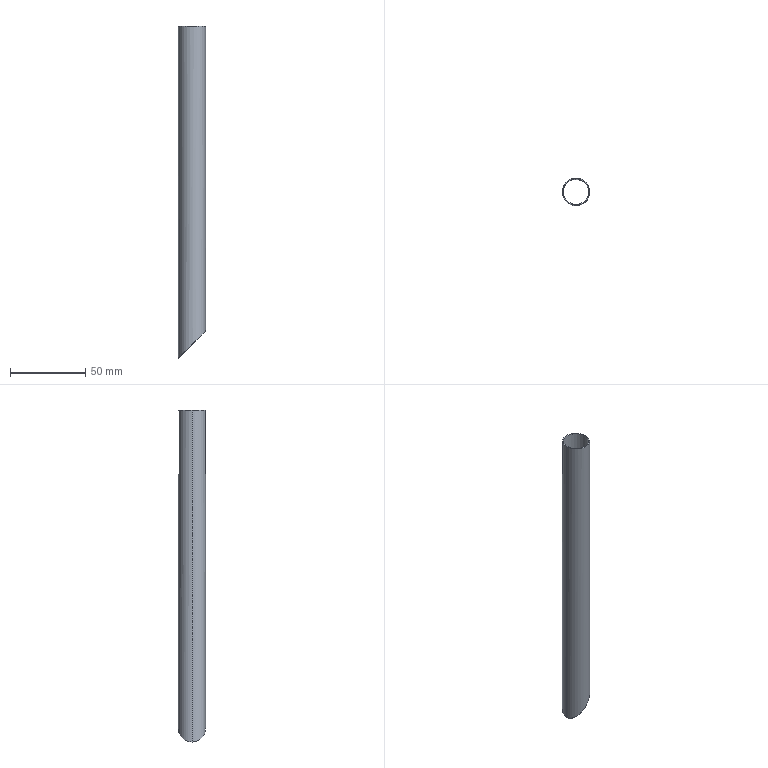Part | SolidWorks | features Extrusion 1, ICE 1 | 1 solid | 6 faces | box 18 x 18 x 220 mm | volume 5800 mm3 | cylinder 4 | plane 2 | commonest cylinder face diameters 17 x2 18 x2
STEP:
#1=CARTESIAN_POINT('',(-8.5,0.,220.));
#2=VERTEX_POINT('',#1);
#3=CARTESIAN_POINT('',(8.5,0.,220.));
#4=VERTEX_POINT('',#3);
#5=CARTESIAN_POINT('',(0.,0.,220.));
#6=DIRECTION('',(0.,0.,1.));
#7=DIRECTION('',(1.,0.,0.));
#8=AXIS2_PLACEMENT_3D('',#5,#6,#7);
#9=CIRCLE('',#8,8.5);
#10=EDGE_CURVE('',#2,#4,#9,.T.);
#11=ORIENTED_EDGE('',*,*,#10,.T.);
#12=CARTESIAN_POINT('',(8.5,0.,17.5));
#13=VERTEX_POINT('',#12);
#14=CARTESIAN_POINT('',(8.5,0.,220.));
#15=DIRECTION('',(0.,0.,-1.));
#16=VECTOR('',#15,1000.);
#17=LINE('',#14,#16);
#18=EDGE_CURVE('',#4,#13,#17,.T.);
#19=ORIENTED_EDGE('',*,*,#18,.T.);
#20=CARTESIAN_POINT('',(-8.5,0.,0.5));
#21=VERTEX_POINT('',#20);
#22=CARTESIAN_POINT('',(-8.5,0.,0.5));
#23=CARTESIAN_POINT('',(-8.5,-17.,0.5));
#24=CARTESIAN_POINT('',(8.5,-17.,17.5));
#25=CARTESIAN_POINT('',(8.5,0.,17.5));
#26=(BOUNDED_CURVE()B_SPLINE_CURVE(3,(#22,#23,#24,#25),.UNSPECIFIED.,.F.,.F.)B_SPLINE_CURVE_WITH_KNOTS((4,4),(0.,3.142),.UNSPECIFIED.)CURVE()GEOMETRIC_REPRESENTATION_ITEM()RATIONAL_B_SPLINE_CURVE((1.,0.3333,0.3333,1.))REPRESENTATION_ITEM(''));
#27=EDGE_CURVE('',#21,#13,#26,.T.);
#28=ORIENTED_EDGE('',*,*,#27,.F.);
#29=CARTESIAN_POINT('',(-8.5,0.,220.));
#30=DIRECTION('',(0.,0.,-1.));
#31=VECTOR('',#30,1000.);
#32=LINE('',#29,#31);
#33=EDGE_CURVE('',#2,#21,#32,.T.);
#34=ORIENTED_EDGE('',*,*,#33,.F.);
#35=EDGE_LOOP('',(#11,#19,#28,#34));
#36=FACE_OUTER_BOUND('',#35,.T.);
#37=CARTESIAN_POINT('',(0.,0.,220.));
#38=DIRECTION('',(0.,0.,-1.));
#39=DIRECTION('',(-1.,0.,0.));
#40=AXIS2_PLACEMENT_3D('',#37,#38,#39);
#41=CYLINDRICAL_SURFACE('',#40,8.5);
#42=ADVANCED_FACE('',(#36),#41,.F.);
#43=CARTESIAN_POINT('',(9.,0.,220.));
#44=VERTEX_POINT('',#43);
#45=CARTESIAN_POINT('',(-9.,0.,220.));
#46=VERTEX_POINT('',#45);
#47=CARTESIAN_POINT('',(0.,0.,220.));
#48=DIRECTION('',(0.,0.,1.));
#49=DIRECTION('',(1.,0.,0.));
#50=AXIS2_PLACEMENT_3D('',#47,#48,#49);
#51=CIRCLE('',#50,9.);
#52=EDGE_CURVE('',#44,#46,#51,.T.);
#53=ORIENTED_EDGE('',*,*,#52,.F.);
#54=CARTESIAN_POINT('',(9.,0.,18.));
#55=VERTEX_POINT('',#54);
#56=CARTESIAN_POINT('',(9.,0.,220.));
#57=DIRECTION('',(0.,0.,-1.));
#58=VECTOR('',#57,1000.);
#59=LINE('',#56,#58);
#60=EDGE_CURVE('',#44,#55,#59,.T.);
#61=ORIENTED_EDGE('',*,*,#60,.T.);
#62=CARTESIAN_POINT('',(-9.,0.,0.));
#63=VERTEX_POINT('',#62);
#64=CARTESIAN_POINT('',(9.,0.,18.));
#65=CARTESIAN_POINT('',(9.,18.,18.));
#66=CARTESIAN_POINT('',(-9.,18.,0.));
#67=CARTESIAN_POINT('',(-9.,0.,0.));
#68=(BOUNDED_CURVE()B_SPLINE_CURVE(3,(#64,#65,#66,#67),.UNSPECIFIED.,.F.,.F.)B_SPLINE_CURVE_WITH_KNOTS((4,4),(3.142,6.283),.UNSPECIFIED.)CURVE()GEOMETRIC_REPRESENTATION_ITEM()RATIONAL_B_SPLINE_CURVE((1.,0.3333,0.3333,1.))REPRESENTATION_ITEM(''));
#69=EDGE_CURVE('',#55,#63,#68,.T.);
#70=ORIENTED_EDGE('',*,*,#69,.T.);
#71=CARTESIAN_POINT('',(-9.,0.,220.));
#72=DIRECTION('',(0.,0.,-1.));
#73=VECTOR('',#72,1000.);
#74=LINE('',#71,#73);
#75=EDGE_CURVE('',#46,#63,#74,.T.);
#76=ORIENTED_EDGE('',*,*,#75,.F.);
#77=EDGE_LOOP('',(#53,#61,#70,#76));
#78=FACE_OUTER_BOUND('',#77,.T.);
#79=CARTESIAN_POINT('',(0.,0.,220.));
#80=DIRECTION('',(0.,0.,-1.));
#81=DIRECTION('',(-1.,0.,0.));
#82=AXIS2_PLACEMENT_3D('',#79,#80,#81);
#83=CYLINDRICAL_SURFACE('',#82,9.);
#84=ADVANCED_FACE('',(#78),#83,.T.);
#85=CARTESIAN_POINT('',(0.,0.,220.));
#86=DIRECTION('',(0.,0.,1.));
#87=DIRECTION('',(1.,0.,0.));
#88=AXIS2_PLACEMENT_3D('',#85,#86,#87);
#89=CIRCLE('',#88,9.);
#90=EDGE_CURVE('',#46,#44,#89,.T.);
#91=ORIENTED_EDGE('',*,*,#90,.T.);
#92=ORIENTED_EDGE('',*,*,#52,.T.);
#93=EDGE_LOOP('',(#91,#92));
#94=FACE_OUTER_BOUND('',#93,.T.);
#95=ORIENTED_EDGE('',*,*,#10,.F.);
#96=CARTESIAN_POINT('',(0.,0.,220.));
#97=DIRECTION('',(0.,0.,1.));
#98=DIRECTION('',(1.,0.,0.));
#99=AXIS2_PLACEMENT_3D('',#96,#97,#98);
#100=CIRCLE('',#99,8.5);
#101=EDGE_CURVE('',#4,#2,#100,.T.);
#102=ORIENTED_EDGE('',*,*,#101,.F.);
#103=EDGE_LOOP('',(#95,#102));
#104=FACE_BOUND('',#103,.T.);
#105=CARTESIAN_POINT('',(0.,0.,220.));
#106=DIRECTION('',(0.,0.,1.));
#107=DIRECTION('',(1.,0.,0.));
#108=AXIS2_PLACEMENT_3D('',#105,#106,#107);
#109=PLANE('',#108);
#110=ADVANCED_FACE('',(#94,#104),#109,.T.);
#111=ORIENTED_EDGE('',*,*,#60,.F.);
#112=ORIENTED_EDGE('',*,*,#90,.F.);
#113=ORIENTED_EDGE('',*,*,#75,.T.);
#114=CARTESIAN_POINT('',(-9.,0.,0.));
#115=CARTESIAN_POINT('',(-9.,-18.,0.));
#116=CARTESIAN_POINT('',(9.,-18.,18.));
#117=CARTESIAN_POINT('',(9.,0.,18.));
#118=(BOUNDED_CURVE()B_SPLINE_CURVE(3,(#114,#115,#116,#117),.UNSPECIFIED.,.F.,.F.)B_SPLINE_CURVE_WITH_KNOTS((4,4),(0.,3.142),.UNSPECIFIED.)CURVE()GEOMETRIC_REPRESENTATION_ITEM()RATIONAL_B_SPLINE_CURVE((1.,0.3333,0.3333,1.))REPRESENTATION_ITEM(''));
#119=EDGE_CURVE('',#63,#55,#118,.T.);
#120=ORIENTED_EDGE('',*,*,#119,.T.);
#121=EDGE_LOOP('',(#111,#112,#113,#120));
#122=FACE_OUTER_BOUND('',#121,.T.);
#123=CARTESIAN_POINT('',(0.,0.,220.));
#124=DIRECTION('',(0.,0.,-1.));
#125=DIRECTION('',(-1.,0.,0.));
#126=AXIS2_PLACEMENT_3D('',#123,#124,#125);
#127=CYLINDRICAL_SURFACE('',#126,9.);
#128=ADVANCED_FACE('',(#122),#127,.T.);
#129=ORIENTED_EDGE('',*,*,#18,.F.);
#130=ORIENTED_EDGE('',*,*,#101,.T.);
#131=ORIENTED_EDGE('',*,*,#33,.T.);
#132=CARTESIAN_POINT('',(8.5,0.,17.5));
#133=CARTESIAN_POINT('',(8.5,17.,17.5));
#134=CARTESIAN_POINT('',(-8.5,17.,0.5));
#135=CARTESIAN_POINT('',(-8.5,0.,0.5));
#136=(BOUNDED_CURVE()B_SPLINE_CURVE(3,(#132,#133,#134,#135),.UNSPECIFIED.,.F.,.F.)B_SPLINE_CURVE_WITH_KNOTS((4,4),(3.142,6.283),.UNSPECIFIED.)CURVE()GEOMETRIC_REPRESENTATION_ITEM()RATIONAL_B_SPLINE_CURVE((1.,0.3333,0.3333,1.))REPRESENTATION_ITEM(''));
#137=EDGE_CURVE('',#13,#21,#136,.T.);
#138=ORIENTED_EDGE('',*,*,#137,.F.);
#139=EDGE_LOOP('',(#129,#130,#131,#138));
#140=FACE_OUTER_BOUND('',#139,.T.);
#141=CARTESIAN_POINT('',(0.,0.,220.));
#142=DIRECTION('',(0.,0.,-1.));
#143=DIRECTION('',(-1.,0.,0.));
#144=AXIS2_PLACEMENT_3D('',#141,#142,#143);
#145=CYLINDRICAL_SURFACE('',#144,8.5);
#146=ADVANCED_FACE('',(#140),#145,.F.);
#147=ORIENTED_EDGE('',*,*,#27,.T.);
#148=ORIENTED_EDGE('',*,*,#137,.T.);
#149=EDGE_LOOP('',(#147,#148));
#150=FACE_BOUND('',#149,.T.);
#151=ORIENTED_EDGE('',*,*,#119,.F.);
#152=ORIENTED_EDGE('',*,*,#69,.F.);
#153=EDGE_LOOP('',(#151,#152));
#154=FACE_OUTER_BOUND('',#153,.T.);
#155=CARTESIAN_POINT('',(-9.,-110.,0.));
#156=DIRECTION('',(-0.7071,0.,0.7071));
#157=DIRECTION('',(0.7071,0.,0.7071));
#158=AXIS2_PLACEMENT_3D('',#155,#156,#157);
#159=PLANE('',#158);
#160=ADVANCED_FACE('',(#150,#154),#159,.F.);
#161=CLOSED_SHELL('',(#42,#84,#110,#128,#146,#160));
#162=MANIFOLD_SOLID_BREP('',#161);
#163=CARTESIAN_POINT('',(0.,0.,0.));
#164=DIRECTION('',(0.,0.,1.));
#165=DIRECTION('',(1.,0.,0.));
#166=AXIS2_PLACEMENT_3D('',#163,#164,#165);
#167=(LENGTH_UNIT()NAMED_UNIT(*)SI_UNIT(.MILLI.,.METRE.));
#168=UNCERTAINTY_MEASURE_WITH_UNIT(LENGTH_MEASURE(0.00001),#167,'','');
#169=(NAMED_UNIT(*)PLANE_ANGLE_UNIT()SI_UNIT($,.RADIAN.));
#170=(NAMED_UNIT(*)SI_UNIT($,.STERADIAN.)SOLID_ANGLE_UNIT());
#171=(GEOMETRIC_REPRESENTATION_CONTEXT(3)GLOBAL_UNCERTAINTY_ASSIGNED_CONTEXT((#168))GLOBAL_UNIT_ASSIGNED_CONTEXT((#167,#169,#170))REPRESENTATION_CONTEXT('',''));
#172=ADVANCED_BREP_SHAPE_REPRESENTATION('',(#162,#166),#171);